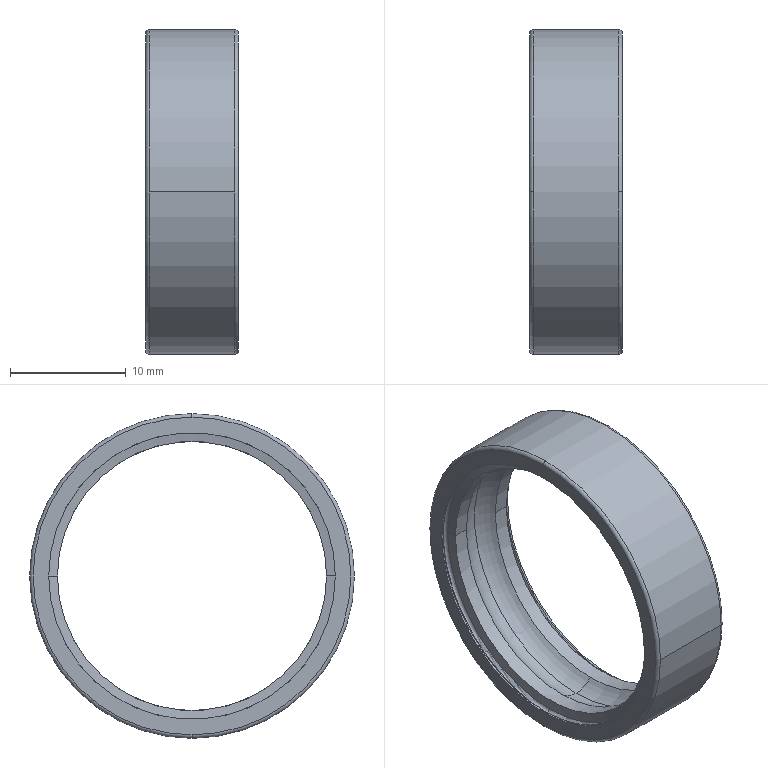Part | SolidWorks | features BaseBody 1 | 1 solid | 32 faces | box 8 x 28 x 28 mm | volume 1280 mm3 | torus 16 | cylinder 10 | cone 4 | plane 2 | commonest cylinder face diameters 23.2 x4 24.72 x4 28 x2
STEP:
#1=CARTESIAN_POINT('',(7.544,0.,-12.664));
#2=VERTEX_POINT('',#1);
#3=CARTESIAN_POINT('',(7.544,0.,12.664));
#4=VERTEX_POINT('',#3);
#5=CARTESIAN_POINT('',(7.544,0.,0.));
#6=DIRECTION('',(1.,0.,0.));
#7=DIRECTION('',(0.,0.,1.));
#8=AXIS2_PLACEMENT_3D('',#5,#6,#7);
#9=CIRCLE('',#8,12.664);
#10=EDGE_CURVE('',#2,#4,#9,.T.);
#11=ORIENTED_EDGE('',*,*,#10,.T.);
#12=CARTESIAN_POINT('',(7.245,0.,12.413));
#13=VERTEX_POINT('',#12);
#14=CARTESIAN_POINT('',(7.544,0.,12.36));
#15=DIRECTION('',(0.,-1.,0.));
#16=DIRECTION('',(0.,0.,1.));
#17=AXIS2_PLACEMENT_3D('',#14,#15,#16);
#18=CIRCLE('',#17,0.304);
#19=EDGE_CURVE('',#4,#13,#18,.T.);
#20=ORIENTED_EDGE('',*,*,#19,.T.);
#21=CARTESIAN_POINT('',(7.245,12.413,0.));
#22=VERTEX_POINT('',#21);
#23=CARTESIAN_POINT('',(7.245,0.,0.));
#24=DIRECTION('',(1.,0.,0.));
#25=DIRECTION('',(0.,1.,0.));
#26=AXIS2_PLACEMENT_3D('',#23,#24,#25);
#27=CIRCLE('',#26,12.413);
#28=EDGE_CURVE('',#22,#13,#27,.T.);
#29=ORIENTED_EDGE('',*,*,#28,.F.);
#30=CARTESIAN_POINT('',(7.245,0.,-12.413));
#31=VERTEX_POINT('',#30);
#32=CARTESIAN_POINT('',(7.245,0.,0.));
#33=DIRECTION('',(1.,0.,0.));
#34=DIRECTION('',(0.,1.,0.));
#35=AXIS2_PLACEMENT_3D('',#32,#33,#34);
#36=CIRCLE('',#35,12.413);
#37=EDGE_CURVE('',#31,#22,#36,.T.);
#38=ORIENTED_EDGE('',*,*,#37,.F.);
#39=CARTESIAN_POINT('',(7.544,0.,-12.36));
#40=DIRECTION('',(0.,-1.,0.));
#41=DIRECTION('',(0.,0.,-1.));
#42=AXIS2_PLACEMENT_3D('',#39,#40,#41);
#43=CIRCLE('',#42,0.304);
#44=EDGE_CURVE('',#31,#2,#43,.T.);
#45=ORIENTED_EDGE('',*,*,#44,.T.);
#46=EDGE_LOOP('',(#11,#20,#29,#38,#45));
#47=FACE_OUTER_BOUND('',#46,.T.);
#48=CARTESIAN_POINT('',(7.544,0.,0.));
#49=DIRECTION('',(1.,0.,0.));
#50=DIRECTION('',(0.,0.,-1.));
#51=AXIS2_PLACEMENT_3D('',#48,#49,#50);
#52=TOROIDAL_SURFACE('',#51,12.36,0.304);
#53=ADVANCED_FACE('',(#47),#52,.F.);
#54=CARTESIAN_POINT('',(7.848,12.36,0.));
#55=VERTEX_POINT('',#54);
#56=CARTESIAN_POINT('',(8.,12.36,0.));
#57=VERTEX_POINT('',#56);
#58=CARTESIAN_POINT('',(7.924,12.36,0.));
#59=DIRECTION('',(1.,0.,0.));
#60=VECTOR('',#59,1000.);
#61=LINE('',#58,#60);
#62=EDGE_CURVE('',#55,#57,#61,.T.);
#63=ORIENTED_EDGE('',*,*,#62,.T.);
#64=CARTESIAN_POINT('',(8.,-12.36,0.));
#65=VERTEX_POINT('',#64);
#66=CARTESIAN_POINT('',(8.,0.,0.));
#67=DIRECTION('',(1.,0.,0.));
#68=DIRECTION('',(0.,1.,0.));
#69=AXIS2_PLACEMENT_3D('',#66,#67,#68);
#70=CIRCLE('',#69,12.36);
#71=EDGE_CURVE('',#57,#65,#70,.T.);
#72=ORIENTED_EDGE('',*,*,#71,.T.);
#73=CARTESIAN_POINT('',(7.848,-12.36,0.));
#74=VERTEX_POINT('',#73);
#75=CARTESIAN_POINT('',(7.924,-12.36,0.));
#76=DIRECTION('',(-1.,0.,0.));
#77=VECTOR('',#76,1000.);
#78=LINE('',#75,#77);
#79=EDGE_CURVE('',#65,#74,#78,.T.);
#80=ORIENTED_EDGE('',*,*,#79,.T.);
#81=CARTESIAN_POINT('',(7.848,0.,12.36));
#82=VERTEX_POINT('',#81);
#83=CARTESIAN_POINT('',(7.848,0.,0.));
#84=DIRECTION('',(1.,0.,0.));
#85=DIRECTION('',(0.,1.,0.));
#86=AXIS2_PLACEMENT_3D('',#83,#84,#85);
#87=CIRCLE('',#86,12.36);
#88=EDGE_CURVE('',#82,#74,#87,.T.);
#89=ORIENTED_EDGE('',*,*,#88,.F.);
#90=CARTESIAN_POINT('',(7.848,0.,0.));
#91=DIRECTION('',(1.,0.,0.));
#92=DIRECTION('',(0.,1.,0.));
#93=AXIS2_PLACEMENT_3D('',#90,#91,#92);
#94=CIRCLE('',#93,12.36);
#95=EDGE_CURVE('',#55,#82,#94,.T.);
#96=ORIENTED_EDGE('',*,*,#95,.F.);
#97=EDGE_LOOP('',(#63,#72,#80,#89,#96));
#98=FACE_OUTER_BOUND('',#97,.T.);
#99=CARTESIAN_POINT('',(7.924,0.,0.));
#100=DIRECTION('',(1.,0.,0.));
#101=DIRECTION('',(0.,1.,0.));
#102=AXIS2_PLACEMENT_3D('',#99,#100,#101);
#103=CYLINDRICAL_SURFACE('',#102,12.36);
#104=ADVANCED_FACE('',(#98),#103,.F.);
#105=ORIENTED_EDGE('',*,*,#71,.F.);
#106=CARTESIAN_POINT('',(8.,0.,0.));
#107=DIRECTION('',(1.,0.,0.));
#108=DIRECTION('',(0.,1.,0.));
#109=AXIS2_PLACEMENT_3D('',#106,#107,#108);
#110=CIRCLE('',#109,12.36);
#111=EDGE_CURVE('',#65,#57,#110,.T.);
#112=ORIENTED_EDGE('',*,*,#111,.F.);
#113=EDGE_LOOP('',(#105,#112));
#114=FACE_BOUND('',#113,.T.);
#115=CARTESIAN_POINT('',(8.,0.,13.7));
#116=VERTEX_POINT('',#115);
#117=CARTESIAN_POINT('',(8.,0.,-13.7));
#118=VERTEX_POINT('',#117);
#119=CARTESIAN_POINT('',(8.,0.,0.));
#120=DIRECTION('',(1.,0.,0.));
#121=DIRECTION('',(0.,1.,0.));
#122=AXIS2_PLACEMENT_3D('',#119,#120,#121);
#123=CIRCLE('',#122,13.7);
#124=EDGE_CURVE('',#116,#118,#123,.T.);
#125=ORIENTED_EDGE('',*,*,#124,.T.);
#126=CARTESIAN_POINT('',(8.,0.,0.));
#127=DIRECTION('',(1.,0.,0.));
#128=DIRECTION('',(0.,1.,0.));
#129=AXIS2_PLACEMENT_3D('',#126,#127,#128);
#130=CIRCLE('',#129,13.7);
#131=EDGE_CURVE('',#118,#116,#130,.T.);
#132=ORIENTED_EDGE('',*,*,#131,.T.);
#133=EDGE_LOOP('',(#125,#132));
#134=FACE_OUTER_BOUND('',#133,.T.);
#135=CARTESIAN_POINT('',(8.,13.03,0.));
#136=DIRECTION('',(1.,0.,0.));
#137=DIRECTION('',(0.,1.,0.));
#138=AXIS2_PLACEMENT_3D('',#135,#136,#137);
#139=PLANE('',#138);
#140=ADVANCED_FACE('',(#114,#134),#139,.T.);
#141=CARTESIAN_POINT('',(7.7,0.,-14.));
#142=VERTEX_POINT('',#141);
#143=CARTESIAN_POINT('',(7.7,0.,-13.7));
#144=DIRECTION('',(0.,-1.,0.));
#145=DIRECTION('',(0.,0.,-1.));
#146=AXIS2_PLACEMENT_3D('',#143,#144,#145);
#147=CIRCLE('',#146,0.3);
#148=EDGE_CURVE('',#142,#118,#147,.T.);
#149=ORIENTED_EDGE('',*,*,#148,.T.);
#150=ORIENTED_EDGE('',*,*,#124,.F.);
#151=CARTESIAN_POINT('',(7.7,0.,14.));
#152=VERTEX_POINT('',#151);
#153=CARTESIAN_POINT('',(7.7,0.,13.7));
#154=DIRECTION('',(0.,-1.,0.));
#155=DIRECTION('',(0.,0.,1.));
#156=AXIS2_PLACEMENT_3D('',#153,#154,#155);
#157=CIRCLE('',#156,0.3);
#158=EDGE_CURVE('',#116,#152,#157,.T.);
#159=ORIENTED_EDGE('',*,*,#158,.T.);
#160=CARTESIAN_POINT('',(7.7,-14.,0.));
#161=VERTEX_POINT('',#160);
#162=CARTESIAN_POINT('',(7.7,0.,0.));
#163=DIRECTION('',(1.,0.,0.));
#164=DIRECTION('',(0.,1.,0.));
#165=AXIS2_PLACEMENT_3D('',#162,#163,#164);
#166=CIRCLE('',#165,14.);
#167=EDGE_CURVE('',#152,#161,#166,.T.);
#168=ORIENTED_EDGE('',*,*,#167,.T.);
#169=CARTESIAN_POINT('',(7.7,0.,0.));
#170=DIRECTION('',(1.,0.,0.));
#171=DIRECTION('',(0.,1.,0.));
#172=AXIS2_PLACEMENT_3D('',#169,#170,#171);
#173=CIRCLE('',#172,14.);
#174=EDGE_CURVE('',#161,#142,#173,.T.);
#175=ORIENTED_EDGE('',*,*,#174,.T.);
#176=EDGE_LOOP('',(#149,#150,#159,#168,#175));
#177=FACE_OUTER_BOUND('',#176,.T.);
#178=CARTESIAN_POINT('',(7.7,0.,0.));
#179=DIRECTION('',(1.,0.,0.));
#180=DIRECTION('',(0.,0.,-1.));
#181=AXIS2_PLACEMENT_3D('',#178,#179,#180);
#182=TOROIDAL_SURFACE('',#181,13.7,0.3);
#183=ADVANCED_FACE('',(#177),#182,.T.);
#184=CARTESIAN_POINT('',(0.3,14.,0.));
#185=VERTEX_POINT('',#184);
#186=CARTESIAN_POINT('',(7.7,14.,0.));
#187=VERTEX_POINT('',#186);
#188=CARTESIAN_POINT('',(4.,14.,0.));
#189=DIRECTION('',(1.,0.,0.));
#190=VECTOR('',#189,1000.);
#191=LINE('',#188,#190);
#192=EDGE_CURVE('',#185,#187,#191,.T.);
#193=ORIENTED_EDGE('',*,*,#192,.T.);
#194=CARTESIAN_POINT('',(7.7,0.,0.));
#195=DIRECTION('',(1.,0.,0.));
#196=DIRECTION('',(0.,1.,0.));
#197=AXIS2_PLACEMENT_3D('',#194,#195,#196);
#198=CIRCLE('',#197,14.);
#199=EDGE_CURVE('',#142,#187,#198,.T.);
#200=ORIENTED_EDGE('',*,*,#199,.F.);
#201=ORIENTED_EDGE('',*,*,#174,.F.);
#202=CARTESIAN_POINT('',(0.3,-14.,0.));
#203=VERTEX_POINT('',#202);
#204=CARTESIAN_POINT('',(4.,-14.,0.));
#205=DIRECTION('',(-1.,0.,0.));
#206=VECTOR('',#205,1000.);
#207=LINE('',#204,#206);
#208=EDGE_CURVE('',#161,#203,#207,.T.);
#209=ORIENTED_EDGE('',*,*,#208,.T.);
#210=CARTESIAN_POINT('',(0.3,0.,-14.));
#211=VERTEX_POINT('',#210);
#212=CARTESIAN_POINT('',(0.3,0.,0.));
#213=DIRECTION('',(1.,0.,0.));
#214=DIRECTION('',(0.,1.,0.));
#215=AXIS2_PLACEMENT_3D('',#212,#213,#214);
#216=CIRCLE('',#215,14.);
#217=EDGE_CURVE('',#203,#211,#216,.T.);
#218=ORIENTED_EDGE('',*,*,#217,.T.);
#219=CARTESIAN_POINT('',(0.3,0.,0.));
#220=DIRECTION('',(1.,0.,0.));
#221=DIRECTION('',(0.,1.,0.));
#222=AXIS2_PLACEMENT_3D('',#219,#220,#221);
#223=CIRCLE('',#222,14.);
#224=EDGE_CURVE('',#211,#185,#223,.T.);
#225=ORIENTED_EDGE('',*,*,#224,.T.);
#226=EDGE_LOOP('',(#193,#200,#201,#209,#218,#225));
#227=FACE_OUTER_BOUND('',#226,.T.);
#228=CARTESIAN_POINT('',(4.,0.,0.));
#229=DIRECTION('',(1.,0.,0.));
#230=DIRECTION('',(0.,1.,0.));
#231=AXIS2_PLACEMENT_3D('',#228,#229,#230);
#232=CYLINDRICAL_SURFACE('',#231,14.);
#233=ADVANCED_FACE('',(#227),#232,.T.);
#234=CARTESIAN_POINT('',(0.,0.,-13.7));
#235=VERTEX_POINT('',#234);
#236=CARTESIAN_POINT('',(0.3,0.,-13.7));
#237=DIRECTION('',(0.,-1.,0.));
#238=DIRECTION('',(0.,0.,-1.));
#239=AXIS2_PLACEMENT_3D('',#236,#237,#238);
#240=CIRCLE('',#239,0.3);
#241=EDGE_CURVE('',#235,#211,#240,.T.);
#242=ORIENTED_EDGE('',*,*,#241,.T.);
#243=ORIENTED_EDGE('',*,*,#217,.F.);
#244=CARTESIAN_POINT('',(0.3,0.,14.));
#245=VERTEX_POINT('',#244);
#246=CARTESIAN_POINT('',(0.3,0.,0.));
#247=DIRECTION('',(1.,0.,0.));
#248=DIRECTION('',(0.,1.,0.));
#249=AXIS2_PLACEMENT_3D('',#246,#247,#248);
#250=CIRCLE('',#249,14.);
#251=EDGE_CURVE('',#245,#203,#250,.T.);
#252=ORIENTED_EDGE('',*,*,#251,.F.);
#253=CARTESIAN_POINT('',(0.,0.,13.7));
#254=VERTEX_POINT('',#253);
#255=CARTESIAN_POINT('',(0.3,0.,13.7));
#256=DIRECTION('',(0.,-1.,0.));
#257=DIRECTION('',(0.,0.,1.));
#258=AXIS2_PLACEMENT_3D('',#255,#256,#257);
#259=CIRCLE('',#258,0.3);
#260=EDGE_CURVE('',#245,#254,#259,.T.);
#261=ORIENTED_EDGE('',*,*,#260,.T.);
#262=CARTESIAN_POINT('',(0.,0.,0.));
#263=DIRECTION('',(1.,0.,0.));
#264=DIRECTION('',(0.,1.,0.));
#265=AXIS2_PLACEMENT_3D('',#262,#263,#264);
#266=CIRCLE('',#265,13.7);
#267=EDGE_CURVE('',#254,#235,#266,.T.);
#268=ORIENTED_EDGE('',*,*,#267,.T.);
#269=EDGE_LOOP('',(#242,#243,#252,#261,#268));
#270=FACE_OUTER_BOUND('',#269,.T.);
#271=CARTESIAN_POINT('',(0.3,0.,0.));
#272=DIRECTION('',(1.,0.,0.));
#273=DIRECTION('',(0.,0.,-1.));
#274=AXIS2_PLACEMENT_3D('',#271,#272,#273);
#275=TOROIDAL_SURFACE('',#274,13.7,0.3);
#276=ADVANCED_FACE('',(#270),#275,.T.);
#277=CARTESIAN_POINT('',(0.,12.36,0.));
#278=VERTEX_POINT('',#277);
#279=CARTESIAN_POINT('',(0.,-12.36,0.));
#280=VERTEX_POINT('',#279);
#281=CARTESIAN_POINT('',(0.,0.,0.));
#282=DIRECTION('',(1.,0.,0.));
#283=DIRECTION('',(0.,1.,0.));
#284=AXIS2_PLACEMENT_3D('',#281,#282,#283);
#285=CIRCLE('',#284,12.36);
#286=EDGE_CURVE('',#278,#280,#285,.T.);
#287=ORIENTED_EDGE('',*,*,#286,.T.);
#288=CARTESIAN_POINT('',(0.,0.,0.));
#289=DIRECTION('',(1.,0.,0.));
#290=DIRECTION('',(0.,1.,0.));
#291=AXIS2_PLACEMENT_3D('',#288,#289,#290);
#292=CIRCLE('',#291,12.36);
#293=EDGE_CURVE('',#280,#278,#292,.T.);
#294=ORIENTED_EDGE('',*,*,#293,.T.);
#295=EDGE_LOOP('',(#287,#294));
#296=FACE_BOUND('',#295,.T.);
#297=CARTESIAN_POINT('',(0.,0.,0.));
#298=DIRECTION('',(1.,0.,0.));
#299=DIRECTION('',(0.,1.,0.));
#300=AXIS2_PLACEMENT_3D('',#297,#298,#299);
#301=CIRCLE('',#300,13.7);
#302=EDGE_CURVE('',#235,#254,#301,.T.);
#303=ORIENTED_EDGE('',*,*,#302,.F.);
#304=ORIENTED_EDGE('',*,*,#267,.F.);
#305=EDGE_LOOP('',(#303,#304));
#306=FACE_OUTER_BOUND('',#305,.T.);
#307=CARTESIAN_POINT('',(0.,13.03,0.));
#308=DIRECTION('',(-1.,0.,0.));
#309=DIRECTION('',(0.,0.,1.));
#310=AXIS2_PLACEMENT_3D('',#307,#308,#309);
#311=PLANE('',#310);
#312=ADVANCED_FACE('',(#296,#306),#311,.T.);
#313=CARTESIAN_POINT('',(0.152,12.36,0.));
#314=VERTEX_POINT('',#313);
#315=CARTESIAN_POINT('',(0.076,12.36,0.));
#316=DIRECTION('',(1.,0.,0.));
#317=VECTOR('',#316,1000.);
#318=LINE('',#315,#317);
#319=EDGE_CURVE('',#278,#314,#318,.T.);
#320=ORIENTED_EDGE('',*,*,#319,.T.);
#321=CARTESIAN_POINT('',(0.152,0.,12.36));
#322=VERTEX_POINT('',#321);
#323=CARTESIAN_POINT('',(0.152,0.,0.));
#324=DIRECTION('',(1.,0.,0.));
#325=DIRECTION('',(0.,1.,0.));
#326=AXIS2_PLACEMENT_3D('',#323,#324,#325);
#327=CIRCLE('',#326,12.36);
#328=EDGE_CURVE('',#314,#322,#327,.T.);
#329=ORIENTED_EDGE('',*,*,#328,.T.);
#330=CARTESIAN_POINT('',(0.152,-12.36,0.));
#331=VERTEX_POINT('',#330);
#332=CARTESIAN_POINT('',(0.152,0.,0.));
#333=DIRECTION('',(1.,0.,0.));
#334=DIRECTION('',(0.,1.,0.));
#335=AXIS2_PLACEMENT_3D('',#332,#333,#334);
#336=CIRCLE('',#335,12.36);
#337=EDGE_CURVE('',#322,#331,#336,.T.);
#338=ORIENTED_EDGE('',*,*,#337,.T.);
#339=CARTESIAN_POINT('',(0.076,-12.36,0.));
#340=DIRECTION('',(-1.,0.,0.));
#341=VECTOR('',#340,1000.);
#342=LINE('',#339,#341);
#343=EDGE_CURVE('',#331,#280,#342,.T.);
#344=ORIENTED_EDGE('',*,*,#343,.T.);
#345=ORIENTED_EDGE('',*,*,#286,.F.);
#346=EDGE_LOOP('',(#320,#329,#338,#344,#345));
#347=FACE_OUTER_BOUND('',#346,.T.);
#348=CARTESIAN_POINT('',(0.076,0.,0.));
#349=DIRECTION('',(1.,0.,0.));
#350=DIRECTION('',(0.,1.,0.));
#351=AXIS2_PLACEMENT_3D('',#348,#349,#350);
#352=CYLINDRICAL_SURFACE('',#351,12.36);
#353=ADVANCED_FACE('',(#347),#352,.F.);
#354=CARTESIAN_POINT('',(0.456,0.,-12.664));
#355=VERTEX_POINT('',#354);
#356=CARTESIAN_POINT('',(0.456,0.,12.664));
#357=VERTEX_POINT('',#356);
#358=CARTESIAN_POINT('',(0.456,0.,0.));
#359=DIRECTION('',(1.,0.,0.));
#360=DIRECTION('',(0.,0.,1.));
#361=AXIS2_PLACEMENT_3D('',#358,#359,#360);
#362=CIRCLE('',#361,12.664);
#363=EDGE_CURVE('',#355,#357,#362,.T.);
#364=ORIENTED_EDGE('',*,*,#363,.T.);
#365=CARTESIAN_POINT('',(0.456,0.,12.36));
#366=DIRECTION('',(0.,-1.,0.));
#367=DIRECTION('',(0.,0.,1.));
#368=AXIS2_PLACEMENT_3D('',#365,#366,#367);
#369=CIRCLE('',#368,0.304);
#370=EDGE_CURVE('',#357,#322,#369,.T.);
#371=ORIENTED_EDGE('',*,*,#370,.T.);
#372=ORIENTED_EDGE('',*,*,#328,.F.);
#373=CARTESIAN_POINT('',(0.152,0.,-12.36));
#374=VERTEX_POINT('',#373);
#375=CARTESIAN_POINT('',(0.152,0.,0.));
#376=DIRECTION('',(1.,0.,0.));
#377=DIRECTION('',(0.,1.,0.));
#378=AXIS2_PLACEMENT_3D('',#375,#376,#377);
#379=CIRCLE('',#378,12.36);
#380=EDGE_CURVE('',#374,#314,#379,.T.);
#381=ORIENTED_EDGE('',*,*,#380,.F.);
#382=CARTESIAN_POINT('',(0.456,0.,-12.36));
#383=DIRECTION('',(0.,-1.,0.));
#384=DIRECTION('',(0.,0.,-1.));
#385=AXIS2_PLACEMENT_3D('',#382,#383,#384);
#386=CIRCLE('',#385,0.304);
#387=EDGE_CURVE('',#374,#355,#386,.T.);
#388=ORIENTED_EDGE('',*,*,#387,.T.);
#389=EDGE_LOOP('',(#364,#371,#372,#381,#388));
#390=FACE_OUTER_BOUND('',#389,.T.);
#391=CARTESIAN_POINT('',(0.456,0.,0.));
#392=DIRECTION('',(1.,0.,0.));
#393=DIRECTION('',(0.,0.,-1.));
#394=AXIS2_PLACEMENT_3D('',#391,#392,#393);
#395=TOROIDAL_SURFACE('',#394,12.36,0.304);
#396=ADVANCED_FACE('',(#390),#395,.F.);
#397=CARTESIAN_POINT('',(0.7554,12.413,0.));
#398=VERTEX_POINT('',#397);
#399=CARTESIAN_POINT('',(0.8987,11.6,0.));
#400=VERTEX_POINT('',#399);
#401=CARTESIAN_POINT('',(0.827,12.006,0.));
#402=DIRECTION('',(0.1736,-0.9848,0.));
#403=VECTOR('',#402,1000.);
#404=LINE('',#401,#403);
#405=EDGE_CURVE('',#398,#400,#404,.T.);
#406=ORIENTED_EDGE('',*,*,#405,.T.);
#407=CARTESIAN_POINT('',(0.8987,-11.6,0.));
#408=VERTEX_POINT('',#407);
#409=CARTESIAN_POINT('',(0.8987,0.,0.));
#410=DIRECTION('',(1.,0.,0.));
#411=DIRECTION('',(0.,1.,0.));
#412=AXIS2_PLACEMENT_3D('',#409,#410,#411);
#413=CIRCLE('',#412,11.6);
#414=EDGE_CURVE('',#400,#408,#413,.T.);
#415=ORIENTED_EDGE('',*,*,#414,.T.);
#416=CARTESIAN_POINT('',(0.7554,-12.413,0.));
#417=VERTEX_POINT('',#416);
#418=CARTESIAN_POINT('',(0.827,-12.006,0.));
#419=DIRECTION('',(-0.1736,-0.9848,0.));
#420=VECTOR('',#419,1000.);
#421=LINE('',#418,#420);
#422=EDGE_CURVE('',#408,#417,#421,.T.);
#423=ORIENTED_EDGE('',*,*,#422,.T.);
#424=CARTESIAN_POINT('',(0.7554,0.,12.413));
#425=VERTEX_POINT('',#424);
#426=CARTESIAN_POINT('',(0.7554,0.,0.));
#427=DIRECTION('',(1.,0.,0.));
#428=DIRECTION('',(0.,1.,0.));
#429=AXIS2_PLACEMENT_3D('',#426,#427,#428);
#430=CIRCLE('',#429,12.413);
#431=EDGE_CURVE('',#425,#417,#430,.T.);
#432=ORIENTED_EDGE('',*,*,#431,.F.);
#433=CARTESIAN_POINT('',(0.7554,0.,0.));
#434=DIRECTION('',(1.,0.,0.));
#435=DIRECTION('',(0.,1.,0.));
#436=AXIS2_PLACEMENT_3D('',#433,#434,#435);
#437=CIRCLE('',#436,12.413);
#438=EDGE_CURVE('',#398,#425,#437,.T.);
#439=ORIENTED_EDGE('',*,*,#438,.F.);
#440=EDGE_LOOP('',(#406,#415,#423,#432,#439));
#441=FACE_OUTER_BOUND('',#440,.T.);
#442=CARTESIAN_POINT('',(0.827,0.,0.));
#443=DIRECTION('',(-1.,0.,0.));
#444=DIRECTION('',(0.,1.,0.));
#445=AXIS2_PLACEMENT_3D('',#442,#443,#444);
#446=CONICAL_SURFACE('',#445,12.006,1.396);
#447=ADVANCED_FACE('',(#441),#446,.F.);
#448=CARTESIAN_POINT('',(2.237,11.6,0.));
#449=VERTEX_POINT('',#448);
#450=CARTESIAN_POINT('',(1.568,11.6,0.));
#451=DIRECTION('',(1.,0.,0.));
#452=VECTOR('',#451,1000.);
#453=LINE('',#450,#452);
#454=EDGE_CURVE('',#400,#449,#453,.T.);
#455=ORIENTED_EDGE('',*,*,#454,.T.);
#456=CARTESIAN_POINT('',(2.237,0.,11.6));
#457=VERTEX_POINT('',#456);
#458=CARTESIAN_POINT('',(2.237,0.,0.));
#459=DIRECTION('',(1.,0.,0.));
#460=DIRECTION('',(0.,1.,0.));
#461=AXIS2_PLACEMENT_3D('',#458,#459,#460);
#462=CIRCLE('',#461,11.6);
#463=EDGE_CURVE('',#449,#457,#462,.T.);
#464=ORIENTED_EDGE('',*,*,#463,.T.);
#465=CARTESIAN_POINT('',(2.237,-11.6,0.));
#466=VERTEX_POINT('',#465);
#467=CARTESIAN_POINT('',(2.237,0.,0.));
#468=DIRECTION('',(1.,0.,0.));
#469=DIRECTION('',(0.,1.,0.));
#470=AXIS2_PLACEMENT_3D('',#467,#468,#469);
#471=CIRCLE('',#470,11.6);
#472=EDGE_CURVE('',#457,#466,#471,.T.);
#473=ORIENTED_EDGE('',*,*,#472,.T.);
#474=CARTESIAN_POINT('',(1.568,-11.6,0.));
#475=DIRECTION('',(-1.,0.,0.));
#476=VECTOR('',#475,1000.);
#477=LINE('',#474,#476);
#478=EDGE_CURVE('',#466,#408,#477,.T.);
#479=ORIENTED_EDGE('',*,*,#478,.T.);
#480=ORIENTED_EDGE('',*,*,#414,.F.);
#481=EDGE_LOOP('',(#455,#464,#473,#479,#480));
#482=FACE_OUTER_BOUND('',#481,.T.);
#483=CARTESIAN_POINT('',(1.568,0.,0.));
#484=DIRECTION('',(1.,0.,0.));
#485=DIRECTION('',(0.,1.,0.));
#486=AXIS2_PLACEMENT_3D('',#483,#484,#485);
#487=CYLINDRICAL_SURFACE('',#486,11.6);
#488=ADVANCED_FACE('',(#482),#487,.F.);
#489=CARTESIAN_POINT('',(4.,0.,-12.381));
#490=VERTEX_POINT('',#489);
#491=CARTESIAN_POINT('',(4.,0.,12.381));
#492=VERTEX_POINT('',#491);
#493=CARTESIAN_POINT('',(4.,0.,0.));
#494=DIRECTION('',(1.,0.,0.));
#495=DIRECTION('',(0.,0.,1.));
#496=AXIS2_PLACEMENT_3D('',#493,#494,#495);
#497=CIRCLE('',#496,12.381);
#498=EDGE_CURVE('',#490,#492,#497,.T.);
#499=ORIENTED_EDGE('',*,*,#498,.T.);
#500=CARTESIAN_POINT('',(4.,0.,10.));
#501=DIRECTION('',(0.,-1.,0.));
#502=DIRECTION('',(0.,0.,1.));
#503=AXIS2_PLACEMENT_3D('',#500,#501,#502);
#504=CIRCLE('',#503,2.381);
#505=EDGE_CURVE('',#492,#457,#504,.T.);
#506=ORIENTED_EDGE('',*,*,#505,.T.);
#507=ORIENTED_EDGE('',*,*,#463,.F.);
#508=CARTESIAN_POINT('',(2.237,0.,-11.6));
#509=VERTEX_POINT('',#508);
#510=CARTESIAN_POINT('',(2.237,0.,0.));
#511=DIRECTION('',(1.,0.,0.));
#512=DIRECTION('',(0.,1.,0.));
#513=AXIS2_PLACEMENT_3D('',#510,#511,#512);
#514=CIRCLE('',#513,11.6);
#515=EDGE_CURVE('',#509,#449,#514,.T.);
#516=ORIENTED_EDGE('',*,*,#515,.F.);
#517=CARTESIAN_POINT('',(4.,0.,-10.));
#518=DIRECTION('',(0.,-1.,0.));
#519=DIRECTION('',(0.,0.,-1.));
#520=AXIS2_PLACEMENT_3D('',#517,#518,#519);
#521=CIRCLE('',#520,2.381);
#522=EDGE_CURVE('',#509,#490,#521,.T.);
#523=ORIENTED_EDGE('',*,*,#522,.T.);
#524=EDGE_LOOP('',(#499,#506,#507,#516,#523));
#525=FACE_OUTER_BOUND('',#524,.T.);
#526=CARTESIAN_POINT('',(4.,0.,0.));
#527=DIRECTION('',(1.,0.,0.));
#528=DIRECTION('',(0.,0.,-1.));
#529=AXIS2_PLACEMENT_3D('',#526,#527,#528);
#530=TOROIDAL_SURFACE('',#529,10.,2.381);
#531=ADVANCED_FACE('',(#525),#530,.F.);
#532=CARTESIAN_POINT('',(5.763,11.6,0.));
#533=VERTEX_POINT('',#532);
#534=CARTESIAN_POINT('',(7.101,11.6,0.));
#535=VERTEX_POINT('',#534);
#536=CARTESIAN_POINT('',(6.432,11.6,0.));
#537=DIRECTION('',(1.,0.,0.));
#538=VECTOR('',#537,1000.);
#539=LINE('',#536,#538);
#540=EDGE_CURVE('',#533,#535,#539,.T.);
#541=ORIENTED_EDGE('',*,*,#540,.T.);
#542=CARTESIAN_POINT('',(7.101,-11.6,0.));
#543=VERTEX_POINT('',#542);
#544=CARTESIAN_POINT('',(7.101,0.,0.));
#545=DIRECTION('',(1.,0.,0.));
#546=DIRECTION('',(0.,1.,0.));
#547=AXIS2_PLACEMENT_3D('',#544,#545,#546);
#548=CIRCLE('',#547,11.6);
#549=EDGE_CURVE('',#535,#543,#548,.T.);
#550=ORIENTED_EDGE('',*,*,#549,.T.);
#551=CARTESIAN_POINT('',(5.763,-11.6,0.));
#552=VERTEX_POINT('',#551);
#553=CARTESIAN_POINT('',(6.432,-11.6,0.));
#554=DIRECTION('',(-1.,0.,0.));
#555=VECTOR('',#554,1000.);
#556=LINE('',#553,#555);
#557=EDGE_CURVE('',#543,#552,#556,.T.);
#558=ORIENTED_EDGE('',*,*,#557,.T.);
#559=CARTESIAN_POINT('',(5.763,0.,11.6));
#560=VERTEX_POINT('',#559);
#561=CARTESIAN_POINT('',(5.763,0.,0.));
#562=DIRECTION('',(1.,0.,0.));
#563=DIRECTION('',(0.,1.,0.));
#564=AXIS2_PLACEMENT_3D('',#561,#562,#563);
#565=CIRCLE('',#564,11.6);
#566=EDGE_CURVE('',#560,#552,#565,.T.);
#567=ORIENTED_EDGE('',*,*,#566,.F.);
#568=CARTESIAN_POINT('',(5.763,0.,0.));
#569=DIRECTION('',(1.,0.,0.));
#570=DIRECTION('',(0.,1.,0.));
#571=AXIS2_PLACEMENT_3D('',#568,#569,#570);
#572=CIRCLE('',#571,11.6);
#573=EDGE_CURVE('',#533,#560,#572,.T.);
#574=ORIENTED_EDGE('',*,*,#573,.F.);
#575=EDGE_LOOP('',(#541,#550,#558,#567,#574));
#576=FACE_OUTER_BOUND('',#575,.T.);
#577=CARTESIAN_POINT('',(6.432,0.,0.));
#578=DIRECTION('',(1.,0.,0.));
#579=DIRECTION('',(0.,1.,0.));
#580=AXIS2_PLACEMENT_3D('',#577,#578,#579);
#581=CYLINDRICAL_SURFACE('',#580,11.6);
#582=ADVANCED_FACE('',(#576),#581,.F.);
#583=CARTESIAN_POINT('',(7.173,12.006,0.));
#584=DIRECTION('',(0.1736,0.9848,0.));
#585=VECTOR('',#584,1000.);
#586=LINE('',#583,#585);
#587=EDGE_CURVE('',#535,#22,#586,.T.);
#588=ORIENTED_EDGE('',*,*,#587,.T.);
#589=ORIENTED_EDGE('',*,*,#28,.T.);
#590=CARTESIAN_POINT('',(7.245,-12.413,0.));
#591=VERTEX_POINT('',#590);
#592=CARTESIAN_POINT('',(7.245,0.,0.));
#593=DIRECTION('',(1.,0.,0.));
#594=DIRECTION('',(0.,1.,0.));
#595=AXIS2_PLACEMENT_3D('',#592,#593,#594);
#596=CIRCLE('',#595,12.413);
#597=EDGE_CURVE('',#13,#591,#596,.T.);
#598=ORIENTED_EDGE('',*,*,#597,.T.);
#599=CARTESIAN_POINT('',(7.173,-12.006,0.));
#600=DIRECTION('',(-0.1736,0.9848,0.));
#601=VECTOR('',#600,1000.);
#602=LINE('',#599,#601);
#603=EDGE_CURVE('',#591,#543,#602,.T.);
#604=ORIENTED_EDGE('',*,*,#603,.T.);
#605=ORIENTED_EDGE('',*,*,#549,.F.);
#606=EDGE_LOOP('',(#588,#589,#598,#604,#605));
#607=FACE_OUTER_BOUND('',#606,.T.);
#608=CARTESIAN_POINT('',(7.173,0.,0.));
#609=DIRECTION('',(1.,0.,0.));
#610=DIRECTION('',(0.,1.,0.));
#611=AXIS2_PLACEMENT_3D('',#608,#609,#610);
#612=CONICAL_SURFACE('',#611,12.006,1.396);
#613=ADVANCED_FACE('',(#607),#612,.F.);
#614=ORIENTED_EDGE('',*,*,#587,.F.);
#615=CARTESIAN_POINT('',(7.101,0.,0.));
#616=DIRECTION('',(1.,0.,0.));
#617=DIRECTION('',(0.,1.,0.));
#618=AXIS2_PLACEMENT_3D('',#615,#616,#617);
#619=CIRCLE('',#618,11.6);
#620=EDGE_CURVE('',#543,#535,#619,.T.);
#621=ORIENTED_EDGE('',*,*,#620,.F.);
#622=ORIENTED_EDGE('',*,*,#603,.F.);
#623=CARTESIAN_POINT('',(7.245,0.,0.));
#624=DIRECTION('',(1.,0.,0.));
#625=DIRECTION('',(0.,1.,0.));
#626=AXIS2_PLACEMENT_3D('',#623,#624,#625);
#627=CIRCLE('',#626,12.413);
#628=EDGE_CURVE('',#591,#31,#627,.T.);
#629=ORIENTED_EDGE('',*,*,#628,.T.);
#630=ORIENTED_EDGE('',*,*,#37,.T.);
#631=EDGE_LOOP('',(#614,#621,#622,#629,#630));
#632=FACE_OUTER_BOUND('',#631,.T.);
#633=CARTESIAN_POINT('',(7.173,0.,0.));
#634=DIRECTION('',(1.,0.,0.));
#635=DIRECTION('',(0.,1.,0.));
#636=AXIS2_PLACEMENT_3D('',#633,#634,#635);
#637=CONICAL_SURFACE('',#636,12.006,1.396);
#638=ADVANCED_FACE('',(#632),#637,.F.);
#639=ORIENTED_EDGE('',*,*,#540,.F.);
#640=CARTESIAN_POINT('',(5.763,0.,-11.6));
#641=VERTEX_POINT('',#640);
#642=CARTESIAN_POINT('',(5.763,0.,0.));
#643=DIRECTION('',(1.,0.,0.));
#644=DIRECTION('',(0.,1.,0.));
#645=AXIS2_PLACEMENT_3D('',#642,#643,#644);
#646=CIRCLE('',#645,11.6);
#647=EDGE_CURVE('',#641,#533,#646,.T.);
#648=ORIENTED_EDGE('',*,*,#647,.F.);
#649=CARTESIAN_POINT('',(5.763,0.,0.));
#650=DIRECTION('',(1.,0.,0.));
#651=DIRECTION('',(0.,1.,0.));
#652=AXIS2_PLACEMENT_3D('',#649,#650,#651);
#653=CIRCLE('',#652,11.6);
#654=EDGE_CURVE('',#552,#641,#653,.T.);
#655=ORIENTED_EDGE('',*,*,#654,.F.);
#656=ORIENTED_EDGE('',*,*,#557,.F.);
#657=ORIENTED_EDGE('',*,*,#620,.T.);
#658=EDGE_LOOP('',(#639,#648,#655,#656,#657));
#659=FACE_OUTER_BOUND('',#658,.T.);
#660=CARTESIAN_POINT('',(6.432,0.,0.));
#661=DIRECTION('',(1.,0.,0.));
#662=DIRECTION('',(0.,1.,0.));
#663=AXIS2_PLACEMENT_3D('',#660,#661,#662);
#664=CYLINDRICAL_SURFACE('',#663,11.6);
#665=ADVANCED_FACE('',(#659),#664,.F.);
#666=CARTESIAN_POINT('',(4.,0.,0.));
#667=DIRECTION('',(1.,0.,0.));
#668=DIRECTION('',(0.,0.,1.));
#669=AXIS2_PLACEMENT_3D('',#666,#667,#668);
#670=CIRCLE('',#669,12.381);
#671=EDGE_CURVE('',#492,#490,#670,.T.);
#672=ORIENTED_EDGE('',*,*,#671,.T.);
#673=ORIENTED_EDGE('',*,*,#522,.F.);
#674=CARTESIAN_POINT('',(2.237,0.,0.));
#675=DIRECTION('',(1.,0.,0.));
#676=DIRECTION('',(0.,1.,0.));
#677=AXIS2_PLACEMENT_3D('',#674,#675,#676);
#678=CIRCLE('',#677,11.6);
#679=EDGE_CURVE('',#466,#509,#678,.T.);
#680=ORIENTED_EDGE('',*,*,#679,.F.);
#681=ORIENTED_EDGE('',*,*,#472,.F.);
#682=ORIENTED_EDGE('',*,*,#505,.F.);
#683=EDGE_LOOP('',(#672,#673,#680,#681,#682));
#684=FACE_OUTER_BOUND('',#683,.T.);
#685=CARTESIAN_POINT('',(4.,0.,0.));
#686=DIRECTION('',(1.,0.,0.));
#687=DIRECTION('',(0.,0.,-1.));
#688=AXIS2_PLACEMENT_3D('',#685,#686,#687);
#689=TOROIDAL_SURFACE('',#688,10.,2.381);
#690=ADVANCED_FACE('',(#684),#689,.F.);
#691=ORIENTED_EDGE('',*,*,#454,.F.);
#692=CARTESIAN_POINT('',(0.8987,0.,0.));
#693=DIRECTION('',(1.,0.,0.));
#694=DIRECTION('',(0.,1.,0.));
#695=AXIS2_PLACEMENT_3D('',#692,#693,#694);
#696=CIRCLE('',#695,11.6);
#697=EDGE_CURVE('',#408,#400,#696,.T.);
#698=ORIENTED_EDGE('',*,*,#697,.F.);
#699=ORIENTED_EDGE('',*,*,#478,.F.);
#700=ORIENTED_EDGE('',*,*,#679,.T.);
#701=ORIENTED_EDGE('',*,*,#515,.T.);
#702=EDGE_LOOP('',(#691,#698,#699,#700,#701));
#703=FACE_OUTER_BOUND('',#702,.T.);
#704=CARTESIAN_POINT('',(1.568,0.,0.));
#705=DIRECTION('',(1.,0.,0.));
#706=DIRECTION('',(0.,1.,0.));
#707=AXIS2_PLACEMENT_3D('',#704,#705,#706);
#708=CYLINDRICAL_SURFACE('',#707,11.6);
#709=ADVANCED_FACE('',(#703),#708,.F.);
#710=ORIENTED_EDGE('',*,*,#405,.F.);
#711=CARTESIAN_POINT('',(0.7554,0.,-12.413));
#712=VERTEX_POINT('',#711);
#713=CARTESIAN_POINT('',(0.7554,0.,0.));
#714=DIRECTION('',(1.,0.,0.));
#715=DIRECTION('',(0.,1.,0.));
#716=AXIS2_PLACEMENT_3D('',#713,#714,#715);
#717=CIRCLE('',#716,12.413);
#718=EDGE_CURVE('',#712,#398,#717,.T.);
#719=ORIENTED_EDGE('',*,*,#718,.F.);
#720=CARTESIAN_POINT('',(0.7554,0.,0.));
#721=DIRECTION('',(1.,0.,0.));
#722=DIRECTION('',(0.,1.,0.));
#723=AXIS2_PLACEMENT_3D('',#720,#721,#722);
#724=CIRCLE('',#723,12.413);
#725=EDGE_CURVE('',#417,#712,#724,.T.);
#726=ORIENTED_EDGE('',*,*,#725,.F.);
#727=ORIENTED_EDGE('',*,*,#422,.F.);
#728=ORIENTED_EDGE('',*,*,#697,.T.);
#729=EDGE_LOOP('',(#710,#719,#726,#727,#728));
#730=FACE_OUTER_BOUND('',#729,.T.);
#731=CARTESIAN_POINT('',(0.827,0.,0.));
#732=DIRECTION('',(-1.,0.,0.));
#733=DIRECTION('',(0.,1.,0.));
#734=AXIS2_PLACEMENT_3D('',#731,#732,#733);
#735=CONICAL_SURFACE('',#734,12.006,1.396);
#736=ADVANCED_FACE('',(#730),#735,.F.);
#737=CARTESIAN_POINT('',(0.456,0.,0.));
#738=DIRECTION('',(1.,0.,0.));
#739=DIRECTION('',(0.,0.,1.));
#740=AXIS2_PLACEMENT_3D('',#737,#738,#739);
#741=CIRCLE('',#740,12.664);
#742=EDGE_CURVE('',#357,#355,#741,.T.);
#743=ORIENTED_EDGE('',*,*,#742,.T.);
#744=ORIENTED_EDGE('',*,*,#387,.F.);
#745=CARTESIAN_POINT('',(0.152,0.,0.));
#746=DIRECTION('',(1.,0.,0.));
#747=DIRECTION('',(0.,1.,0.));
#748=AXIS2_PLACEMENT_3D('',#745,#746,#747);
#749=CIRCLE('',#748,12.36);
#750=EDGE_CURVE('',#331,#374,#749,.T.);
#751=ORIENTED_EDGE('',*,*,#750,.F.);
#752=ORIENTED_EDGE('',*,*,#337,.F.);
#753=ORIENTED_EDGE('',*,*,#370,.F.);
#754=EDGE_LOOP('',(#743,#744,#751,#752,#753));
#755=FACE_OUTER_BOUND('',#754,.T.);
#756=CARTESIAN_POINT('',(0.456,0.,0.));
#757=DIRECTION('',(1.,0.,0.));
#758=DIRECTION('',(0.,0.,-1.));
#759=AXIS2_PLACEMENT_3D('',#756,#757,#758);
#760=TOROIDAL_SURFACE('',#759,12.36,0.304);
#761=ADVANCED_FACE('',(#755),#760,.F.);
#762=ORIENTED_EDGE('',*,*,#319,.F.);
#763=ORIENTED_EDGE('',*,*,#293,.F.);
#764=ORIENTED_EDGE('',*,*,#343,.F.);
#765=ORIENTED_EDGE('',*,*,#750,.T.);
#766=ORIENTED_EDGE('',*,*,#380,.T.);
#767=EDGE_LOOP('',(#762,#763,#764,#765,#766));
#768=FACE_OUTER_BOUND('',#767,.T.);
#769=CARTESIAN_POINT('',(0.076,0.,0.));
#770=DIRECTION('',(1.,0.,0.));
#771=DIRECTION('',(0.,1.,0.));
#772=AXIS2_PLACEMENT_3D('',#769,#770,#771);
#773=CYLINDRICAL_SURFACE('',#772,12.36);
#774=ADVANCED_FACE('',(#768),#773,.F.);
#775=ORIENTED_EDGE('',*,*,#241,.F.);
#776=ORIENTED_EDGE('',*,*,#302,.T.);
#777=ORIENTED_EDGE('',*,*,#260,.F.);
#778=CARTESIAN_POINT('',(0.3,0.,0.));
#779=DIRECTION('',(1.,0.,0.));
#780=DIRECTION('',(0.,1.,0.));
#781=AXIS2_PLACEMENT_3D('',#778,#779,#780);
#782=CIRCLE('',#781,14.);
#783=EDGE_CURVE('',#185,#245,#782,.T.);
#784=ORIENTED_EDGE('',*,*,#783,.F.);
#785=ORIENTED_EDGE('',*,*,#224,.F.);
#786=EDGE_LOOP('',(#775,#776,#777,#784,#785));
#787=FACE_OUTER_BOUND('',#786,.T.);
#788=CARTESIAN_POINT('',(0.3,0.,0.));
#789=DIRECTION('',(1.,0.,0.));
#790=DIRECTION('',(0.,0.,-1.));
#791=AXIS2_PLACEMENT_3D('',#788,#789,#790);
#792=TOROIDAL_SURFACE('',#791,13.7,0.3);
#793=ADVANCED_FACE('',(#787),#792,.T.);
#794=ORIENTED_EDGE('',*,*,#192,.F.);
#795=ORIENTED_EDGE('',*,*,#783,.T.);
#796=ORIENTED_EDGE('',*,*,#251,.T.);
#797=ORIENTED_EDGE('',*,*,#208,.F.);
#798=ORIENTED_EDGE('',*,*,#167,.F.);
#799=CARTESIAN_POINT('',(7.7,0.,0.));
#800=DIRECTION('',(1.,0.,0.));
#801=DIRECTION('',(0.,1.,0.));
#802=AXIS2_PLACEMENT_3D('',#799,#800,#801);
#803=CIRCLE('',#802,14.);
#804=EDGE_CURVE('',#187,#152,#803,.T.);
#805=ORIENTED_EDGE('',*,*,#804,.F.);
#806=EDGE_LOOP('',(#794,#795,#796,#797,#798,#805));
#807=FACE_OUTER_BOUND('',#806,.T.);
#808=CARTESIAN_POINT('',(4.,0.,0.));
#809=DIRECTION('',(1.,0.,0.));
#810=DIRECTION('',(0.,1.,0.));
#811=AXIS2_PLACEMENT_3D('',#808,#809,#810);
#812=CYLINDRICAL_SURFACE('',#811,14.);
#813=ADVANCED_FACE('',(#807),#812,.T.);
#814=ORIENTED_EDGE('',*,*,#148,.F.);
#815=ORIENTED_EDGE('',*,*,#199,.T.);
#816=ORIENTED_EDGE('',*,*,#804,.T.);
#817=ORIENTED_EDGE('',*,*,#158,.F.);
#818=ORIENTED_EDGE('',*,*,#131,.F.);
#819=EDGE_LOOP('',(#814,#815,#816,#817,#818));
#820=FACE_OUTER_BOUND('',#819,.T.);
#821=CARTESIAN_POINT('',(7.7,0.,0.));
#822=DIRECTION('',(1.,0.,0.));
#823=DIRECTION('',(0.,0.,-1.));
#824=AXIS2_PLACEMENT_3D('',#821,#822,#823);
#825=TOROIDAL_SURFACE('',#824,13.7,0.3);
#826=ADVANCED_FACE('',(#820),#825,.T.);
#827=ORIENTED_EDGE('',*,*,#62,.F.);
#828=CARTESIAN_POINT('',(7.848,0.,-12.36));
#829=VERTEX_POINT('',#828);
#830=CARTESIAN_POINT('',(7.848,0.,0.));
#831=DIRECTION('',(1.,0.,0.));
#832=DIRECTION('',(0.,1.,0.));
#833=AXIS2_PLACEMENT_3D('',#830,#831,#832);
#834=CIRCLE('',#833,12.36);
#835=EDGE_CURVE('',#829,#55,#834,.T.);
#836=ORIENTED_EDGE('',*,*,#835,.F.);
#837=CARTESIAN_POINT('',(7.848,0.,0.));
#838=DIRECTION('',(1.,0.,0.));
#839=DIRECTION('',(0.,1.,0.));
#840=AXIS2_PLACEMENT_3D('',#837,#838,#839);
#841=CIRCLE('',#840,12.36);
#842=EDGE_CURVE('',#74,#829,#841,.T.);
#843=ORIENTED_EDGE('',*,*,#842,.F.);
#844=ORIENTED_EDGE('',*,*,#79,.F.);
#845=ORIENTED_EDGE('',*,*,#111,.T.);
#846=EDGE_LOOP('',(#827,#836,#843,#844,#845));
#847=FACE_OUTER_BOUND('',#846,.T.);
#848=CARTESIAN_POINT('',(7.924,0.,0.));
#849=DIRECTION('',(1.,0.,0.));
#850=DIRECTION('',(0.,1.,0.));
#851=AXIS2_PLACEMENT_3D('',#848,#849,#850);
#852=CYLINDRICAL_SURFACE('',#851,12.36);
#853=ADVANCED_FACE('',(#847),#852,.F.);
#854=CARTESIAN_POINT('',(7.544,0.,0.));
#855=DIRECTION('',(1.,0.,0.));
#856=DIRECTION('',(0.,0.,1.));
#857=AXIS2_PLACEMENT_3D('',#854,#855,#856);
#858=CIRCLE('',#857,12.664);
#859=EDGE_CURVE('',#4,#2,#858,.T.);
#860=ORIENTED_EDGE('',*,*,#859,.T.);
#861=ORIENTED_EDGE('',*,*,#44,.F.);
#862=ORIENTED_EDGE('',*,*,#628,.F.);
#863=ORIENTED_EDGE('',*,*,#597,.F.);
#864=ORIENTED_EDGE('',*,*,#19,.F.);
#865=EDGE_LOOP('',(#860,#861,#862,#863,#864));
#866=FACE_OUTER_BOUND('',#865,.T.);
#867=CARTESIAN_POINT('',(7.544,0.,0.));
#868=DIRECTION('',(1.,0.,0.));
#869=DIRECTION('',(0.,0.,-1.));
#870=AXIS2_PLACEMENT_3D('',#867,#868,#869);
#871=TOROIDAL_SURFACE('',#870,12.36,0.304);
#872=ADVANCED_FACE('',(#866),#871,.F.);
#873=ORIENTED_EDGE('',*,*,#859,.F.);
#874=CARTESIAN_POINT('',(7.544,0.,12.36));
#875=DIRECTION('',(0.,-1.,0.));
#876=DIRECTION('',(0.,0.,1.));
#877=AXIS2_PLACEMENT_3D('',#874,#875,#876);
#878=CIRCLE('',#877,0.304);
#879=EDGE_CURVE('',#82,#4,#878,.T.);
#880=ORIENTED_EDGE('',*,*,#879,.F.);
#881=ORIENTED_EDGE('',*,*,#88,.T.);
#882=ORIENTED_EDGE('',*,*,#842,.T.);
#883=CARTESIAN_POINT('',(7.544,0.,-12.36));
#884=DIRECTION('',(0.,-1.,0.));
#885=DIRECTION('',(0.,0.,-1.));
#886=AXIS2_PLACEMENT_3D('',#883,#884,#885);
#887=CIRCLE('',#886,0.304);
#888=EDGE_CURVE('',#2,#829,#887,.T.);
#889=ORIENTED_EDGE('',*,*,#888,.F.);
#890=EDGE_LOOP('',(#873,#880,#881,#882,#889));
#891=FACE_OUTER_BOUND('',#890,.T.);
#892=CARTESIAN_POINT('',(7.544,0.,0.));
#893=DIRECTION('',(1.,0.,0.));
#894=DIRECTION('',(0.,0.,-1.));
#895=AXIS2_PLACEMENT_3D('',#892,#893,#894);
#896=TOROIDAL_SURFACE('',#895,12.36,0.304);
#897=ADVANCED_FACE('',(#891),#896,.F.);
#898=ORIENTED_EDGE('',*,*,#742,.F.);
#899=CARTESIAN_POINT('',(0.456,0.,12.36));
#900=DIRECTION('',(0.,-1.,0.));
#901=DIRECTION('',(0.,0.,1.));
#902=AXIS2_PLACEMENT_3D('',#899,#900,#901);
#903=CIRCLE('',#902,0.304);
#904=EDGE_CURVE('',#425,#357,#903,.T.);
#905=ORIENTED_EDGE('',*,*,#904,.F.);
#906=ORIENTED_EDGE('',*,*,#431,.T.);
#907=ORIENTED_EDGE('',*,*,#725,.T.);
#908=CARTESIAN_POINT('',(0.456,0.,-12.36));
#909=DIRECTION('',(0.,-1.,0.));
#910=DIRECTION('',(0.,0.,-1.));
#911=AXIS2_PLACEMENT_3D('',#908,#909,#910);
#912=CIRCLE('',#911,0.304);
#913=EDGE_CURVE('',#355,#712,#912,.T.);
#914=ORIENTED_EDGE('',*,*,#913,.F.);
#915=EDGE_LOOP('',(#898,#905,#906,#907,#914));
#916=FACE_OUTER_BOUND('',#915,.T.);
#917=CARTESIAN_POINT('',(0.456,0.,0.));
#918=DIRECTION('',(1.,0.,0.));
#919=DIRECTION('',(0.,0.,-1.));
#920=AXIS2_PLACEMENT_3D('',#917,#918,#919);
#921=TOROIDAL_SURFACE('',#920,12.36,0.304);
#922=ADVANCED_FACE('',(#916),#921,.F.);
#923=ORIENTED_EDGE('',*,*,#671,.F.);
#924=CARTESIAN_POINT('',(4.,0.,10.));
#925=DIRECTION('',(0.,-1.,0.));
#926=DIRECTION('',(0.,0.,1.));
#927=AXIS2_PLACEMENT_3D('',#924,#925,#926);
#928=CIRCLE('',#927,2.381);
#929=EDGE_CURVE('',#560,#492,#928,.T.);
#930=ORIENTED_EDGE('',*,*,#929,.F.);
#931=ORIENTED_EDGE('',*,*,#566,.T.);
#932=ORIENTED_EDGE('',*,*,#654,.T.);
#933=CARTESIAN_POINT('',(4.,0.,-10.));
#934=DIRECTION('',(0.,-1.,0.));
#935=DIRECTION('',(0.,0.,-1.));
#936=AXIS2_PLACEMENT_3D('',#933,#934,#935);
#937=CIRCLE('',#936,2.381);
#938=EDGE_CURVE('',#490,#641,#937,.T.);
#939=ORIENTED_EDGE('',*,*,#938,.F.);
#940=EDGE_LOOP('',(#923,#930,#931,#932,#939));
#941=FACE_OUTER_BOUND('',#940,.T.);
#942=CARTESIAN_POINT('',(4.,0.,0.));
#943=DIRECTION('',(1.,0.,0.));
#944=DIRECTION('',(0.,0.,-1.));
#945=AXIS2_PLACEMENT_3D('',#942,#943,#944);
#946=TOROIDAL_SURFACE('',#945,10.,2.381);
#947=ADVANCED_FACE('',(#941),#946,.F.);
#948=ORIENTED_EDGE('',*,*,#498,.F.);
#949=ORIENTED_EDGE('',*,*,#938,.T.);
#950=ORIENTED_EDGE('',*,*,#647,.T.);
#951=ORIENTED_EDGE('',*,*,#573,.T.);
#952=ORIENTED_EDGE('',*,*,#929,.T.);
#953=EDGE_LOOP('',(#948,#949,#950,#951,#952));
#954=FACE_OUTER_BOUND('',#953,.T.);
#955=CARTESIAN_POINT('',(4.,0.,0.));
#956=DIRECTION('',(1.,0.,0.));
#957=DIRECTION('',(0.,0.,-1.));
#958=AXIS2_PLACEMENT_3D('',#955,#956,#957);
#959=TOROIDAL_SURFACE('',#958,10.,2.381);
#960=ADVANCED_FACE('',(#954),#959,.F.);
#961=ORIENTED_EDGE('',*,*,#363,.F.);
#962=ORIENTED_EDGE('',*,*,#913,.T.);
#963=ORIENTED_EDGE('',*,*,#718,.T.);
#964=ORIENTED_EDGE('',*,*,#438,.T.);
#965=ORIENTED_EDGE('',*,*,#904,.T.);
#966=EDGE_LOOP('',(#961,#962,#963,#964,#965));
#967=FACE_OUTER_BOUND('',#966,.T.);
#968=CARTESIAN_POINT('',(0.456,0.,0.));
#969=DIRECTION('',(1.,0.,0.));
#970=DIRECTION('',(0.,0.,-1.));
#971=AXIS2_PLACEMENT_3D('',#968,#969,#970);
#972=TOROIDAL_SURFACE('',#971,12.36,0.304);
#973=ADVANCED_FACE('',(#967),#972,.F.);
#974=ORIENTED_EDGE('',*,*,#10,.F.);
#975=ORIENTED_EDGE('',*,*,#888,.T.);
#976=ORIENTED_EDGE('',*,*,#835,.T.);
#977=ORIENTED_EDGE('',*,*,#95,.T.);
#978=ORIENTED_EDGE('',*,*,#879,.T.);
#979=EDGE_LOOP('',(#974,#975,#976,#977,#978));
#980=FACE_OUTER_BOUND('',#979,.T.);
#981=CARTESIAN_POINT('',(7.544,0.,0.));
#982=DIRECTION('',(1.,0.,0.));
#983=DIRECTION('',(0.,0.,-1.));
#984=AXIS2_PLACEMENT_3D('',#981,#982,#983);
#985=TOROIDAL_SURFACE('',#984,12.36,0.304);
#986=ADVANCED_FACE('',(#980),#985,.F.);
#987=CLOSED_SHELL('',(#53,#104,#140,#183,#233,#276,#312,#353,#396,#447,#488,#531,#582,#613,#638,#665,#690,#709,#736,#761,#774,#793,#813,#826,#853,#872,#897,#922,#947,#960,#973,#986));
#988=MANIFOLD_SOLID_BREP('',#987);
#989=CARTESIAN_POINT('',(0.,0.,0.));
#990=DIRECTION('',(0.,0.,1.));
#991=DIRECTION('',(1.,0.,0.));
#992=AXIS2_PLACEMENT_3D('',#989,#990,#991);
#993=(LENGTH_UNIT()NAMED_UNIT(*)SI_UNIT(.MILLI.,.METRE.));
#994=UNCERTAINTY_MEASURE_WITH_UNIT(LENGTH_MEASURE(0.00001),#993,'','');
#995=(NAMED_UNIT(*)PLANE_ANGLE_UNIT()SI_UNIT($,.RADIAN.));
#996=(NAMED_UNIT(*)SI_UNIT($,.STERADIAN.)SOLID_ANGLE_UNIT());
#997=(GEOMETRIC_REPRESENTATION_CONTEXT(3)GLOBAL_UNCERTAINTY_ASSIGNED_CONTEXT((#994))GLOBAL_UNIT_ASSIGNED_CONTEXT((#993,#995,#996))REPRESENTATION_CONTEXT('',''));
#998=ADVANCED_BREP_SHAPE_REPRESENTATION('',(#988,#992),#997);